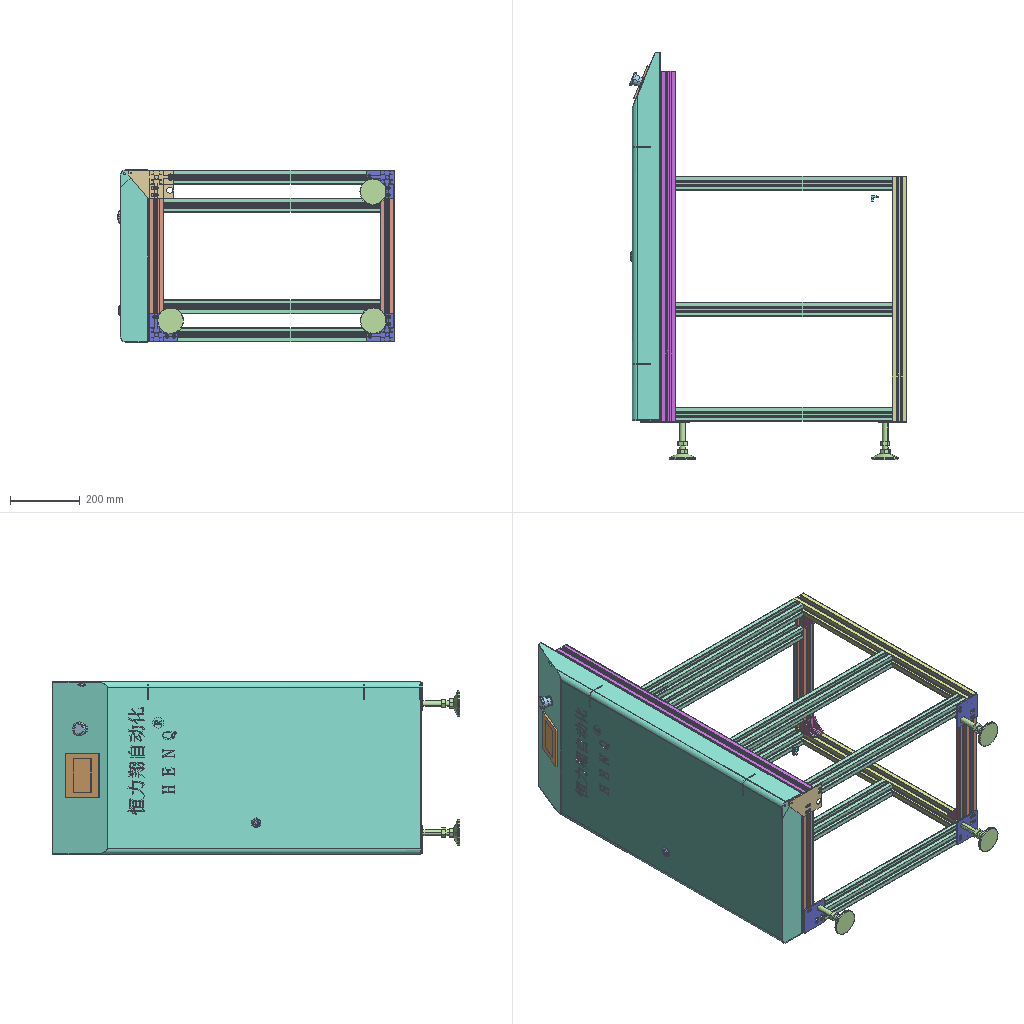Assembly | SolidWorks | 23 different items | 48 placed | box 791 x 1165 x 493 mm
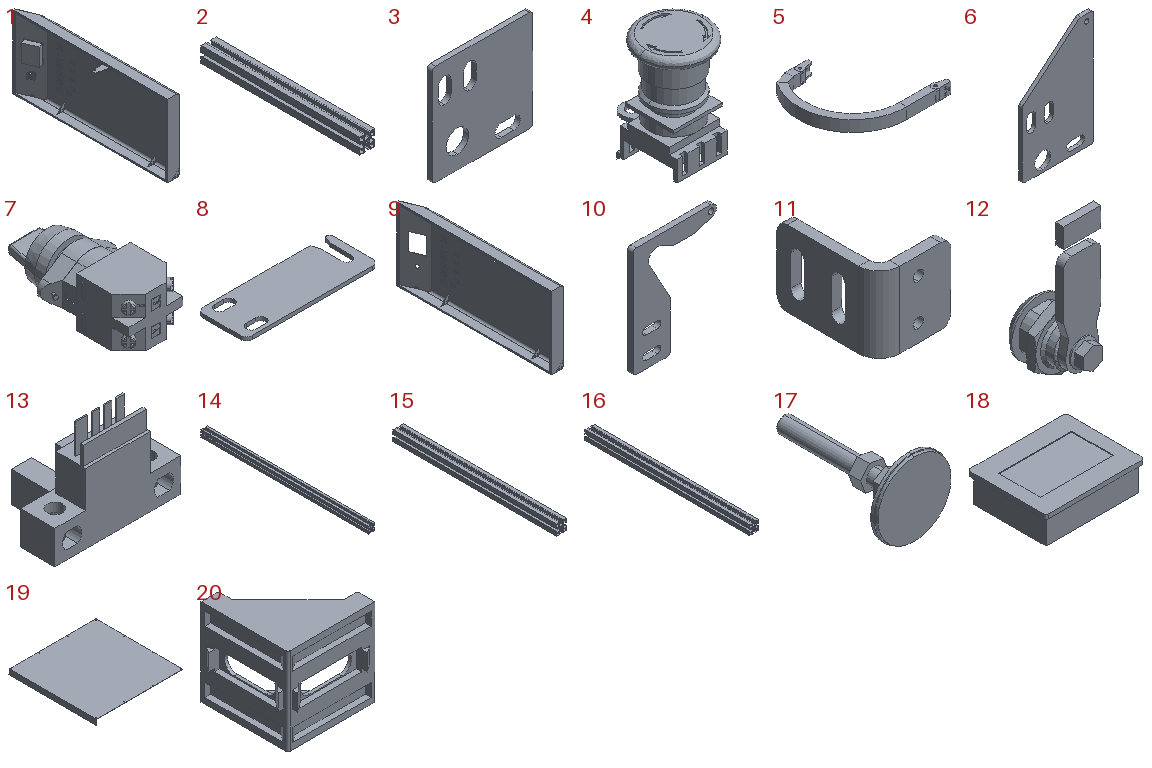Parts list (item | name | quantity | parent item | size | volume | features):
1 | (subassembly) | x1 | - | 127.543 x 1053 x 493 mm | 1598886 mm3 | features AEMSimFeature 1, MirrorCompFeat 1
2 | - | x4 | - | 40 x 410 x 40 mm | 106924 mm3 | features MirrorPattern 2, Extrusion 1
3 | - | x3 | - | 80 x 4 x 80 mm | 22409 mm3 | features Extrusion 1, Fillet 1
4 | - | x1 | in 1 | 40 x 46.376 x 67.3 mm | 38156 mm3 | features BaseBody 3
5 | - | x1 | - | 308.75 x 283.5 x 35 mm | 208341 mm3 | features ICE 8, MirrorPattern 1, Sweep 1
6 | - | x1 | - | 80 x 4 x 130 mm | 31186 mm3 | features ExtruRefSurface 1, Extrusion 1, Fillet 1
7 | - | x1 | - | 44 x 78 x 29 mm | 50843 mm3 | features ICE 14, MirrorPattern 4, Fillet 2, Revolution 2, Chamfer 1, PLine 1, SmartComponentFeature 1
8 | - | x1 | in 1 | 108 x 40 x 3 mm | 11505 mm3 | features Fillet 2, Extrusion 1, HoleWzd 1
9 | - | x1 | in 1 | 80 x 1053 x 493 mm | 1093617 mm3 | features ICE 11, Fillet 2, Cut 1, HoleWzd 1, Shell 1
10 | - | x1 | - | 76 x 5 x 100 mm | 16067 mm3 | features Extrusion 1, Fillet 1
11 | - | x1 | - | 35 x 50 x 37 mm | 12594 mm3 | features EdgeFlange 1, Fillet 1, FlatPattern 1, HoleWzd 1, ICE 1, SMBaseFlange 1, SheetMetal 1
12 | - | x1 | in 1 | 28 x 32 x 75.588 mm | 13581 mm3 | features BaseBody 1, ICE 1, MoveCopyBody 1, Split 1
13 | - | x1 | - | 26.2 x 15.5 x 20.7 mm | 2180 mm3 | features BaseBody 1
14 | - | x2 | - | 40 x 1000 x 40 mm | 260790 mm3 | features MirrorPattern 2, Extrusion 1
15 | - | x8 | - | 40 x 620 x 40 mm | 161690 mm3 | features MirrorPattern 2, Extrusion 1
16 | - | x2 | - | 40 x 700 x 40 mm | 182553 mm3 | features MirrorPattern 2, Extrusion 1
17 | - | x4 | - | 75 x 130 x 75 mm | 80922 mm3 | features Boss 2, Chamfer 1, Revolution 1
18 | - | x1 | in 1 | 128 x 105 x 38.5 mm | 442026 mm3 | features ICE 4, Extrusion 1, Fillet 1
19 | - | x2 | - | 703 x 704 x 40 mm | 781813 mm3 | features HoleWzd 2, EdgeFlange 1, Fillet 1, FlatPattern 1, SMBaseFlange 1, SheetMetal 1
20 | - | x8 | - | 42.5 x 42.5 x 40 mm | 12926 mm3 | features ICE 7, Extrusion 1, Fillet 1, LPattern 1, MirrorPattern 1
21 | SX671 Block_Plate Stacker | x1 | - | - | - | -
22 | Rear Panel_Plate Stacker | x1 | - | - | - | -
23 | Pneumatic Control Assembly_Plate Stacker (subassembly) | x1 | - | - | - | -
Mates (type | each side: item.copy, entity, surface, feature):
In the top assembly
Coincident | 16.1 face plane Boss-Extrude1 | 14.1 face plane Boss-Extrude1
Coincident | 16.1 face plane Mirror2 | 16.2 face plane Mirror2
DistanceDim | 14.1 face plane Mirror2 | 16.1 face plane Mirror2
Coincident | 16.1 edge | 2.1 face plane Mirror1
Coincident | 16.1 face plane Boss-Extrude1 | 15.1 face plane Mirror2
Coincident | 16.1 face plane Boss-Extrude1 | 15.1 face plane Boss-Extrude1
Parallel | 16.1 face plane Mirror2 | 17.1 face plane Extrude2
Coincident | 16.1 face plane Mirror2 | 20.1 face plane Boss-Extrude1 | 2 times
Coincident | 14.1 face plane Mirror2 | 14.2 face plane Mirror2
DistanceDim | 14.1 face plane Mirror2 | 14.2 face plane Mirror2
Coincident | 14.1 face plane Mirror2 | 15.2 face plane Mirror2
Coincident | 14.1 face plane Boss-Extrude1 | 15.2 face plane Boss-Extrude1
Coincident | 14.1 face plane Mirror2 | 2.2 face plane Boss-Extrude1
Coincident | 14.1 face plane Mirror2 | 2.2 face plane Mirror2
Coincident | 14.1 face plane Boss-Extrude1 | 2.2 face plane Boss-Extrude1
Coincident | 14.1 face plane Mirror2 | 20.2 face plane Boss-Extrude1 | 2 times
Coincident | 14.2 face plane Mirror1 | 16.2 face plane Mirror2
Coincident | 14.2 face plane Mirror1 | 15.3 face plane Mirror1
Coincident | 14.2 face plane Mirror2 | 20.3 face plane Boss-Extrude1
Coincident | 14.2 face plane Boss-Extrude1 | 20.3 face plane Boss-Extrude1
Coincident | 16.2 face plane Mirror2 | 15.4 face plane Mirror2
Coincident | 16.2 face plane Mirror2 | 15.4 face plane Boss-Extrude1
Coincident | 16.2 edge | 3.1 face plane Boss-Extrude1
Coincident | 16.2 face plane Mirror1 | 20.4 face plane Boss-Extrude1 | 2 times
Coincident | 15.2 face plane Boss-Extrude1 | 15.3 face plane Boss-Extrude1
Coincident | 15.2 face plane Mirror1 | 15.3 face plane Boss-Extrude1
Coincident | 15.2 face plane Boss-Extrude1 | 15.5 face plane Boss-Extrude1 | 2 times
Coincident | 15.2 face plane Boss-Extrude1 | 15.6 face plane Boss-Extrude1
Coincident | 15.3 face plane Mirror1 | 15.6 face plane Mirror1
Coincident | 15.5 face plane Mirror2 | 15.6 face plane Mirror2
Coincident | 2.2 face plane Mirror2 | 2.1 face plane Mirror2
Coincident | 2.2 face plane Boss-Extrude1 | 2.1 face plane Boss-Extrude1
Coincident | 2.2 face plane Mirror2 | 20.3 face plane Boss-Extrude1
Coincident | 2.2 face plane Mirror2 | 20.2 face plane Boss-Extrude1
DistanceDim | 2.1 face plane Boss-Extrude1 | 17.1 face plane Revolve1
Coincident | 2.1 face plane Boss-Extrude1 | 3.1 face plane Boss-Extrude1
Coincident | 2.1 face plane Mirror1 | 3.1 face plane Boss-Extrude1
Coincident | 2.1 face plane Mirror2 | 20.1 face plane Boss-Extrude1
Coincident | 2.1 face plane Mirror2 | 20.4 face plane Boss-Extrude1
Coincident | 17.1 face plane Revolve1 | 17.2 face plane Revolve1
Coincident | 17.1 face plane Revolve1 | 17.3 face plane Revolve1
Coincident | 17.1 face plane Revolve1 | 17.4 face plane Revolve1
Concentric | 3.1 face cylinder Boss-Extrude1 | 17.4 face cylinder Revolve1
Symmetric | 14.2 face plane Mirror2 | 16.2 face plane Mirror2 | assembly plane
Symmetric | 15.2 face plane Mirror2 | 15.3 face plane Mirror2 | assembly plane
Coincident | 17.1 face plane Revolve1 | assembly plane
Coincident | 15.3 face plane Boss-Extrude1 | 2.2 face plane Mirror1
Coincident | 16.1 face plane Boss-Extrude1 | 2.1 face plane Mirror1
Parallel | 17.3 face plane Extrude2 | assembly plane
Parallel | 17.2 face plane Extrude1 | assembly plane
Parallel | 17.4 face plane Extrude2 | assembly plane
Coincident | 14.2 face plane Boss-Extrude1 | 15.3 face plane Mirror1
Coincident | 16.2 face plane Boss-Extrude1 | 15.4 face plane Mirror2
Coincident | 15.4 face plane Mirror2 | 15.1 face plane Mirror2
DistanceDim | 15.2 face plane Mirror1 | 15.5 face plane Mirror1
Symmetric | 2.3 face plane Boss-Extrude1 | 2.3 face plane Boss-Extrude1 | assembly plane
Coincident | 16.1 face plane Mirror2 | 2.3 face plane Mirror2
Coincident | 16.1 face plane Boss-Extrude1 | 2.3 face plane Mirror2
Symmetric | 2.4 face plane Boss-Extrude1 | 2.4 face plane Boss-Extrude1 | assembly plane
Coincident | 14.2 face plane Mirror2 | 2.4 face plane Mirror2
Coincident | 15.4 face plane Mirror2 | 2.4 face plane Mirror2
Coincident | 14.1 face plane Mirror2 | 19.1 face plane Edge-Flange1
Coincident | 15.2 face plane Mirror2 | 19.1 face plane Base-Flange1
Coincident | 15.2 face plane Boss-Extrude1 | 19.1 face plane Base-Flange1
Parallel | 7.1 plane | assembly plane
Concentric | 17.1 face cylinder Revolve1 | 3.2 face cylinder Boss-Extrude1
Coincident | assembly plane | assembly plane | 3 times
Coincident | 15.6 face plane Mirror1 | assembly face
DistanceDim | assembly face | 14.2 face plane Mirror2
Parallel | assembly face | assembly plane
DistanceDim | 15.7 face plane Mirror2 | 15.8 face plane Mirror2
Coincident | 15.8 face plane Mirror2 | 15.4 face plane Mirror2
Coincident | 15.7 face plane Mirror2 | 15.1 face plane Mirror2
Symmetric | 15.7 face plane Mirror2 | 15.8 face plane Mirror2 | assembly plane
Coincident | 15.7 face plane Boss-Extrude1 | 15.1 face plane Boss-Extrude1
Coincident | 15.8 face plane Boss-Extrude1 | 15.4 face plane Boss-Extrude1
Width | 15.6 face plane Mirror2 | 15.6 face plane Mirror2 | 5.1 face plane Sweep1 | 5.1 face plane Sweep1
Coincident | 15.6 face plane Mirror2 | 5.1 face plane Sweep1
DistanceDim | 5.1 face plane Boss-Extrude1 | 14.2 face plane Mirror1
Coincident | 15.2 face plane Boss-Extrude1 | 3.3 face plane Boss-Extrude1 | 2 times
Coincident | 2.2 face plane Boss-Extrude1 | 3.3 face plane Boss-Extrude1
Concentric | 17.2 face cylinder Revolve1 | 3.3 face cylinder Boss-Extrude1
Coincident | 15.3 face plane Mirror1 | 6.1 face plane Boss-Extrude1 | 2 times
Concentric | 17.3 face cylinder Revolve1 | 6.1 face cylinder Boss-Extrude1
Concentric | 9.1 face cylinder Ø7.0 (7) Diameter Hole1 | 6.1 face cylinder Boss-Extrude1
Coincident | 14.2 face plane Boss-Extrude1 | 11.1 face plane Edge-Flange1
Coincident | 11.1 face plane Base-Flange1 | 10.1 face plane Boss-Extrude1
Parallel | 11.1 face plane Edge-Flange1 | 10.1 face plane Boss-Extrude1
DistanceDim | 6.1 face plane Boss-Extrude1 | 9.1 face plane Boss-Extrude1
LimitPlanarAngleDim | 2.2 face plane Mirror2 | 9.1 face plane Boss-Extrude1
Concentric | 6.1 face cylinder Boss-Extrude1 | 10.1 face cylinder Boss-Extrude1
DistanceDim | 14.2 face plane Mirror2 | 6.1 face plane Boss-Extrude1
Slot | 11.1 face cylinder M6 Tapped Hole1 | 10.1 face plane Boss-Extrude1
Coincident | 14.2 face plane Mirror1 | 19.2 face plane Base-Flange1
Coincident | 14.2 face plane Mirror2 | 19.2 face plane Edge-Flange1
Coincident | 15.3 face plane Mirror1 | 19.2 face plane Base-Flange1
In subassembly 1
Coincident | 8.1 face plane Boss-Extrude1 | 12.1 face plane Imported1 | 2 times
Coincident | 12.1 face plane Imported1 | 9.2 face plane Boss-Extrude1
Concentric | 12.1 face cylinder Imported1 | 9.2 face cylinder Cut-Extrude2
Parallel | 8.1 face plane Boss-Extrude1 | 9.2 face plane Boss-Extrude1
Concentric | 9.2 face cylinder Cut-Extrude4 | 4.1 face cylinder Imported6
Coincident | 9.2 face plane Cut-Extrude3 | 4.1 face plane Imported6
Parallel | 9.2 edge | 4.1 face plane Imported3
Coincident | 9.2 face plane Cut-Extrude4 | 18.1 face plane Boss-Extrude2 | 2 times
Coincident | 9.2 face plane Cut-Extrude3 | 18.1 face plane Boss-Extrude1
DistanceDim | 8.1 face plane Boss-Extrude1 | 12.1 face plane Imported1